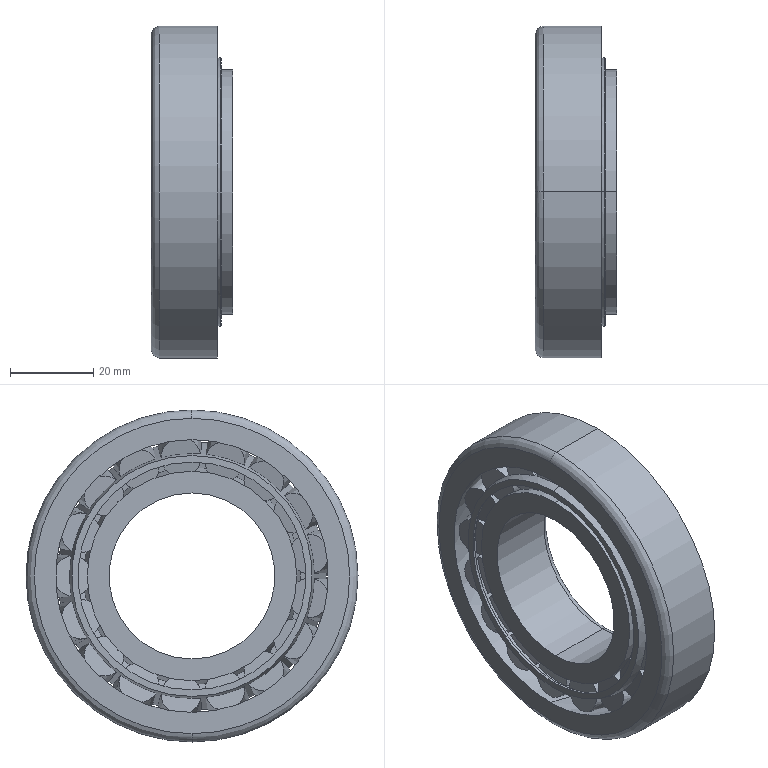Part | STEP file | 30208V11 | 3 solids | 153 faces | box 19.75 x 80 x 80 mm | volume 51729 mm3 | plane 74 | cone 67 | cylinder 8 | torus 4 | commonest cylinder face diameters 40 x2 50.5 x2 58.9 x2 80 x2